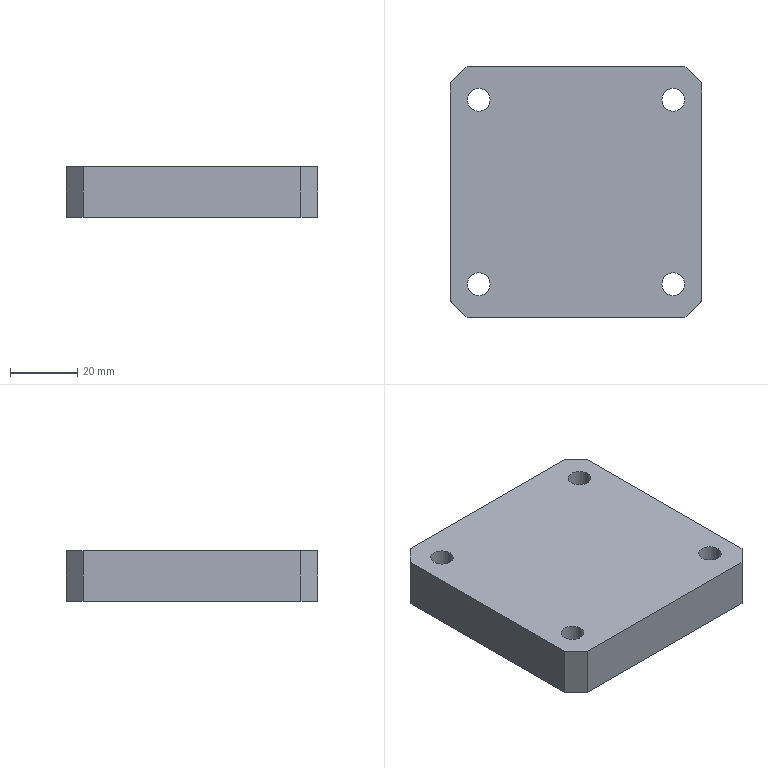Part | SolidWorks | features Extrusion 1, HoleWzd 1 | 1 solid | 18 faces | box 75 x 75 x 15 mm | volume 81446 mm3 | plane 10 | cylinder 8 | commonest cylinder face diameters 6.8 x8
STEP:
#1=CARTESIAN_POINT('',(-25.6,27.5,0.));
#2=VERTEX_POINT('',#1);
#3=CARTESIAN_POINT('',(-32.4,27.5,0.));
#4=VERTEX_POINT('',#3);
#5=CARTESIAN_POINT('',(-29.,27.5,0.));
#6=DIRECTION('',(0.,0.,-1.));
#7=DIRECTION('',(-1.,0.,0.));
#8=AXIS2_PLACEMENT_3D('',#5,#6,#7);
#9=CIRCLE('',#8,3.4);
#10=EDGE_CURVE('',#2,#4,#9,.T.);
#11=ORIENTED_EDGE('',*,*,#10,.T.);
#12=CARTESIAN_POINT('',(-32.4,27.5,15.));
#13=VERTEX_POINT('',#12);
#14=CARTESIAN_POINT('',(-32.4,27.5,15.));
#15=DIRECTION('',(0.,0.,1.));
#16=VECTOR('',#15,1000.);
#17=LINE('',#14,#16);
#18=EDGE_CURVE('',#4,#13,#17,.T.);
#19=ORIENTED_EDGE('',*,*,#18,.T.);
#20=CARTESIAN_POINT('',(-25.6,27.5,15.));
#21=VERTEX_POINT('',#20);
#22=CARTESIAN_POINT('',(-29.,27.5,15.));
#23=DIRECTION('',(0.,0.,1.));
#24=DIRECTION('',(1.,0.,0.));
#25=AXIS2_PLACEMENT_3D('',#22,#23,#24);
#26=CIRCLE('',#25,3.4);
#27=EDGE_CURVE('',#13,#21,#26,.T.);
#28=ORIENTED_EDGE('',*,*,#27,.T.);
#29=CARTESIAN_POINT('',(-25.6,27.5,15.));
#30=DIRECTION('',(0.,0.,1.));
#31=VECTOR('',#30,1000.);
#32=LINE('',#29,#31);
#33=EDGE_CURVE('',#2,#21,#32,.T.);
#34=ORIENTED_EDGE('',*,*,#33,.F.);
#35=EDGE_LOOP('',(#11,#19,#28,#34));
#36=FACE_OUTER_BOUND('',#35,.T.);
#37=CARTESIAN_POINT('',(-29.,27.5,15.));
#38=DIRECTION('',(0.,0.,1.));
#39=DIRECTION('',(1.,0.,0.));
#40=AXIS2_PLACEMENT_3D('',#37,#38,#39);
#41=CYLINDRICAL_SURFACE('',#40,3.4);
#42=ADVANCED_FACE('',(#36),#41,.F.);
#43=CARTESIAN_POINT('',(32.4,27.5,0.));
#44=VERTEX_POINT('',#43);
#45=CARTESIAN_POINT('',(25.6,27.5,0.));
#46=VERTEX_POINT('',#45);
#47=CARTESIAN_POINT('',(29.,27.5,0.));
#48=DIRECTION('',(0.,0.,-1.));
#49=DIRECTION('',(-1.,0.,0.));
#50=AXIS2_PLACEMENT_3D('',#47,#48,#49);
#51=CIRCLE('',#50,3.4);
#52=EDGE_CURVE('',#44,#46,#51,.T.);
#53=ORIENTED_EDGE('',*,*,#52,.T.);
#54=CARTESIAN_POINT('',(25.6,27.5,15.));
#55=VERTEX_POINT('',#54);
#56=CARTESIAN_POINT('',(25.6,27.5,15.));
#57=DIRECTION('',(0.,0.,1.));
#58=VECTOR('',#57,1000.);
#59=LINE('',#56,#58);
#60=EDGE_CURVE('',#46,#55,#59,.T.);
#61=ORIENTED_EDGE('',*,*,#60,.T.);
#62=CARTESIAN_POINT('',(32.4,27.5,15.));
#63=VERTEX_POINT('',#62);
#64=CARTESIAN_POINT('',(29.,27.5,15.));
#65=DIRECTION('',(0.,0.,1.));
#66=DIRECTION('',(1.,0.,0.));
#67=AXIS2_PLACEMENT_3D('',#64,#65,#66);
#68=CIRCLE('',#67,3.4);
#69=EDGE_CURVE('',#55,#63,#68,.T.);
#70=ORIENTED_EDGE('',*,*,#69,.T.);
#71=CARTESIAN_POINT('',(32.4,27.5,15.));
#72=DIRECTION('',(0.,0.,1.));
#73=VECTOR('',#72,1000.);
#74=LINE('',#71,#73);
#75=EDGE_CURVE('',#44,#63,#74,.T.);
#76=ORIENTED_EDGE('',*,*,#75,.F.);
#77=EDGE_LOOP('',(#53,#61,#70,#76));
#78=FACE_OUTER_BOUND('',#77,.T.);
#79=CARTESIAN_POINT('',(29.,27.5,15.));
#80=DIRECTION('',(0.,0.,1.));
#81=DIRECTION('',(1.,0.,0.));
#82=AXIS2_PLACEMENT_3D('',#79,#80,#81);
#83=CYLINDRICAL_SURFACE('',#82,3.4);
#84=ADVANCED_FACE('',(#78),#83,.F.);
#85=CARTESIAN_POINT('',(32.4,-27.5,0.));
#86=VERTEX_POINT('',#85);
#87=CARTESIAN_POINT('',(25.6,-27.5,0.));
#88=VERTEX_POINT('',#87);
#89=CARTESIAN_POINT('',(29.,-27.5,0.));
#90=DIRECTION('',(0.,0.,-1.));
#91=DIRECTION('',(-1.,0.,0.));
#92=AXIS2_PLACEMENT_3D('',#89,#90,#91);
#93=CIRCLE('',#92,3.4);
#94=EDGE_CURVE('',#86,#88,#93,.T.);
#95=ORIENTED_EDGE('',*,*,#94,.T.);
#96=CARTESIAN_POINT('',(25.6,-27.5,15.));
#97=VERTEX_POINT('',#96);
#98=CARTESIAN_POINT('',(25.6,-27.5,15.));
#99=DIRECTION('',(0.,0.,1.));
#100=VECTOR('',#99,1000.);
#101=LINE('',#98,#100);
#102=EDGE_CURVE('',#88,#97,#101,.T.);
#103=ORIENTED_EDGE('',*,*,#102,.T.);
#104=CARTESIAN_POINT('',(32.4,-27.5,15.));
#105=VERTEX_POINT('',#104);
#106=CARTESIAN_POINT('',(29.,-27.5,15.));
#107=DIRECTION('',(0.,0.,1.));
#108=DIRECTION('',(1.,0.,0.));
#109=AXIS2_PLACEMENT_3D('',#106,#107,#108);
#110=CIRCLE('',#109,3.4);
#111=EDGE_CURVE('',#97,#105,#110,.T.);
#112=ORIENTED_EDGE('',*,*,#111,.T.);
#113=CARTESIAN_POINT('',(32.4,-27.5,15.));
#114=DIRECTION('',(0.,0.,1.));
#115=VECTOR('',#114,1000.);
#116=LINE('',#113,#115);
#117=EDGE_CURVE('',#86,#105,#116,.T.);
#118=ORIENTED_EDGE('',*,*,#117,.F.);
#119=EDGE_LOOP('',(#95,#103,#112,#118));
#120=FACE_OUTER_BOUND('',#119,.T.);
#121=CARTESIAN_POINT('',(29.,-27.5,15.));
#122=DIRECTION('',(0.,0.,1.));
#123=DIRECTION('',(1.,0.,0.));
#124=AXIS2_PLACEMENT_3D('',#121,#122,#123);
#125=CYLINDRICAL_SURFACE('',#124,3.4);
#126=ADVANCED_FACE('',(#120),#125,.F.);
#127=CARTESIAN_POINT('',(-25.6,-27.5,0.));
#128=VERTEX_POINT('',#127);
#129=CARTESIAN_POINT('',(-32.4,-27.5,0.));
#130=VERTEX_POINT('',#129);
#131=CARTESIAN_POINT('',(-29.,-27.5,0.));
#132=DIRECTION('',(0.,0.,-1.));
#133=DIRECTION('',(-1.,0.,0.));
#134=AXIS2_PLACEMENT_3D('',#131,#132,#133);
#135=CIRCLE('',#134,3.4);
#136=EDGE_CURVE('',#128,#130,#135,.T.);
#137=ORIENTED_EDGE('',*,*,#136,.T.);
#138=CARTESIAN_POINT('',(-32.4,-27.5,15.));
#139=VERTEX_POINT('',#138);
#140=CARTESIAN_POINT('',(-32.4,-27.5,15.));
#141=DIRECTION('',(0.,0.,1.));
#142=VECTOR('',#141,1000.);
#143=LINE('',#140,#142);
#144=EDGE_CURVE('',#130,#139,#143,.T.);
#145=ORIENTED_EDGE('',*,*,#144,.T.);
#146=CARTESIAN_POINT('',(-25.6,-27.5,15.));
#147=VERTEX_POINT('',#146);
#148=CARTESIAN_POINT('',(-29.,-27.5,15.));
#149=DIRECTION('',(0.,0.,1.));
#150=DIRECTION('',(1.,0.,0.));
#151=AXIS2_PLACEMENT_3D('',#148,#149,#150);
#152=CIRCLE('',#151,3.4);
#153=EDGE_CURVE('',#139,#147,#152,.T.);
#154=ORIENTED_EDGE('',*,*,#153,.T.);
#155=CARTESIAN_POINT('',(-25.6,-27.5,15.));
#156=DIRECTION('',(0.,0.,1.));
#157=VECTOR('',#156,1000.);
#158=LINE('',#155,#157);
#159=EDGE_CURVE('',#128,#147,#158,.T.);
#160=ORIENTED_EDGE('',*,*,#159,.F.);
#161=EDGE_LOOP('',(#137,#145,#154,#160));
#162=FACE_OUTER_BOUND('',#161,.T.);
#163=CARTESIAN_POINT('',(-29.,-27.5,15.));
#164=DIRECTION('',(0.,0.,1.));
#165=DIRECTION('',(1.,0.,0.));
#166=AXIS2_PLACEMENT_3D('',#163,#164,#165);
#167=CYLINDRICAL_SURFACE('',#166,3.4);
#168=ADVANCED_FACE('',(#162),#167,.F.);
#169=CARTESIAN_POINT('',(32.5,37.5,0.));
#170=VERTEX_POINT('',#169);
#171=CARTESIAN_POINT('',(-32.5,37.5,0.));
#172=VERTEX_POINT('',#171);
#173=CARTESIAN_POINT('',(-32.5,37.5,0.));
#174=DIRECTION('',(-1.,0.,0.));
#175=VECTOR('',#174,1000.);
#176=LINE('',#173,#175);
#177=EDGE_CURVE('',#170,#172,#176,.T.);
#178=ORIENTED_EDGE('',*,*,#177,.T.);
#179=CARTESIAN_POINT('',(-32.5,37.5,15.));
#180=VERTEX_POINT('',#179);
#181=CARTESIAN_POINT('',(-32.5,37.5,15.));
#182=DIRECTION('',(0.,0.,-1.));
#183=VECTOR('',#182,1000.);
#184=LINE('',#181,#183);
#185=EDGE_CURVE('',#180,#172,#184,.T.);
#186=ORIENTED_EDGE('',*,*,#185,.F.);
#187=CARTESIAN_POINT('',(32.5,37.5,15.));
#188=VERTEX_POINT('',#187);
#189=CARTESIAN_POINT('',(-32.5,37.5,15.));
#190=DIRECTION('',(-1.,0.,0.));
#191=VECTOR('',#190,1000.);
#192=LINE('',#189,#191);
#193=EDGE_CURVE('',#188,#180,#192,.T.);
#194=ORIENTED_EDGE('',*,*,#193,.F.);
#195=CARTESIAN_POINT('',(32.5,37.5,15.));
#196=DIRECTION('',(0.,0.,-1.));
#197=VECTOR('',#196,1000.);
#198=LINE('',#195,#197);
#199=EDGE_CURVE('',#188,#170,#198,.T.);
#200=ORIENTED_EDGE('',*,*,#199,.T.);
#201=EDGE_LOOP('',(#178,#186,#194,#200));
#202=FACE_OUTER_BOUND('',#201,.T.);
#203=CARTESIAN_POINT('',(-32.5,37.5,15.));
#204=DIRECTION('',(0.,-1.,0.));
#205=DIRECTION('',(0.,0.,-1.));
#206=AXIS2_PLACEMENT_3D('',#203,#204,#205);
#207=PLANE('',#206);
#208=ADVANCED_FACE('',(#202),#207,.F.);
#209=CARTESIAN_POINT('',(-37.5,32.5,0.));
#210=VERTEX_POINT('',#209);
#211=CARTESIAN_POINT('',(-37.5,32.5,0.));
#212=DIRECTION('',(-0.7071,-0.7071,0.));
#213=VECTOR('',#212,1000.);
#214=LINE('',#211,#213);
#215=EDGE_CURVE('',#172,#210,#214,.T.);
#216=ORIENTED_EDGE('',*,*,#215,.T.);
#217=CARTESIAN_POINT('',(-37.5,32.5,15.));
#218=VERTEX_POINT('',#217);
#219=CARTESIAN_POINT('',(-37.5,32.5,15.));
#220=DIRECTION('',(0.,0.,-1.));
#221=VECTOR('',#220,1000.);
#222=LINE('',#219,#221);
#223=EDGE_CURVE('',#218,#210,#222,.T.);
#224=ORIENTED_EDGE('',*,*,#223,.F.);
#225=CARTESIAN_POINT('',(-37.5,32.5,15.));
#226=DIRECTION('',(-0.7071,-0.7071,0.));
#227=VECTOR('',#226,1000.);
#228=LINE('',#225,#227);
#229=EDGE_CURVE('',#180,#218,#228,.T.);
#230=ORIENTED_EDGE('',*,*,#229,.F.);
#231=ORIENTED_EDGE('',*,*,#185,.T.);
#232=EDGE_LOOP('',(#216,#224,#230,#231));
#233=FACE_OUTER_BOUND('',#232,.T.);
#234=CARTESIAN_POINT('',(-37.5,32.5,15.));
#235=DIRECTION('',(0.7071,-0.7071,0.));
#236=DIRECTION('',(0.7071,0.7071,0.));
#237=AXIS2_PLACEMENT_3D('',#234,#235,#236);
#238=PLANE('',#237);
#239=ADVANCED_FACE('',(#233),#238,.F.);
#240=CARTESIAN_POINT('',(-37.5,-32.5,0.));
#241=VERTEX_POINT('',#240);
#242=CARTESIAN_POINT('',(-37.5,32.5,0.));
#243=DIRECTION('',(0.,-1.,0.));
#244=VECTOR('',#243,1000.);
#245=LINE('',#242,#244);
#246=EDGE_CURVE('',#210,#241,#245,.T.);
#247=ORIENTED_EDGE('',*,*,#246,.T.);
#248=CARTESIAN_POINT('',(-37.5,-32.5,15.));
#249=VERTEX_POINT('',#248);
#250=CARTESIAN_POINT('',(-37.5,-32.5,15.));
#251=DIRECTION('',(0.,0.,-1.));
#252=VECTOR('',#251,1000.);
#253=LINE('',#250,#252);
#254=EDGE_CURVE('',#249,#241,#253,.T.);
#255=ORIENTED_EDGE('',*,*,#254,.F.);
#256=CARTESIAN_POINT('',(-37.5,32.5,15.));
#257=DIRECTION('',(0.,-1.,0.));
#258=VECTOR('',#257,1000.);
#259=LINE('',#256,#258);
#260=EDGE_CURVE('',#218,#249,#259,.T.);
#261=ORIENTED_EDGE('',*,*,#260,.F.);
#262=ORIENTED_EDGE('',*,*,#223,.T.);
#263=EDGE_LOOP('',(#247,#255,#261,#262));
#264=FACE_OUTER_BOUND('',#263,.T.);
#265=CARTESIAN_POINT('',(-37.5,32.5,15.));
#266=DIRECTION('',(1.,0.,0.));
#267=DIRECTION('',(0.,0.,-1.));
#268=AXIS2_PLACEMENT_3D('',#265,#266,#267);
#269=PLANE('',#268);
#270=ADVANCED_FACE('',(#264),#269,.F.);
#271=CARTESIAN_POINT('',(-32.5,-37.5,0.));
#272=VERTEX_POINT('',#271);
#273=CARTESIAN_POINT('',(-37.5,-32.5,0.));
#274=DIRECTION('',(0.7071,-0.7071,0.));
#275=VECTOR('',#274,1000.);
#276=LINE('',#273,#275);
#277=EDGE_CURVE('',#241,#272,#276,.T.);
#278=ORIENTED_EDGE('',*,*,#277,.T.);
#279=CARTESIAN_POINT('',(-32.5,-37.5,15.));
#280=VERTEX_POINT('',#279);
#281=CARTESIAN_POINT('',(-32.5,-37.5,15.));
#282=DIRECTION('',(0.,0.,-1.));
#283=VECTOR('',#282,1000.);
#284=LINE('',#281,#283);
#285=EDGE_CURVE('',#280,#272,#284,.T.);
#286=ORIENTED_EDGE('',*,*,#285,.F.);
#287=CARTESIAN_POINT('',(-37.5,-32.5,15.));
#288=DIRECTION('',(0.7071,-0.7071,0.));
#289=VECTOR('',#288,1000.);
#290=LINE('',#287,#289);
#291=EDGE_CURVE('',#249,#280,#290,.T.);
#292=ORIENTED_EDGE('',*,*,#291,.F.);
#293=ORIENTED_EDGE('',*,*,#254,.T.);
#294=EDGE_LOOP('',(#278,#286,#292,#293));
#295=FACE_OUTER_BOUND('',#294,.T.);
#296=CARTESIAN_POINT('',(-37.5,-32.5,15.));
#297=DIRECTION('',(0.7071,0.7071,0.));
#298=DIRECTION('',(-0.7071,0.7071,0.));
#299=AXIS2_PLACEMENT_3D('',#296,#297,#298);
#300=PLANE('',#299);
#301=ADVANCED_FACE('',(#295),#300,.F.);
#302=CARTESIAN_POINT('',(32.5,-37.5,0.));
#303=VERTEX_POINT('',#302);
#304=CARTESIAN_POINT('',(-32.5,-37.5,0.));
#305=DIRECTION('',(1.,0.,0.));
#306=VECTOR('',#305,1000.);
#307=LINE('',#304,#306);
#308=EDGE_CURVE('',#272,#303,#307,.T.);
#309=ORIENTED_EDGE('',*,*,#308,.T.);
#310=CARTESIAN_POINT('',(32.5,-37.5,15.));
#311=VERTEX_POINT('',#310);
#312=CARTESIAN_POINT('',(32.5,-37.5,15.));
#313=DIRECTION('',(0.,0.,-1.));
#314=VECTOR('',#313,1000.);
#315=LINE('',#312,#314);
#316=EDGE_CURVE('',#311,#303,#315,.T.);
#317=ORIENTED_EDGE('',*,*,#316,.F.);
#318=CARTESIAN_POINT('',(-32.5,-37.5,15.));
#319=DIRECTION('',(1.,0.,0.));
#320=VECTOR('',#319,1000.);
#321=LINE('',#318,#320);
#322=EDGE_CURVE('',#280,#311,#321,.T.);
#323=ORIENTED_EDGE('',*,*,#322,.F.);
#324=ORIENTED_EDGE('',*,*,#285,.T.);
#325=EDGE_LOOP('',(#309,#317,#323,#324));
#326=FACE_OUTER_BOUND('',#325,.T.);
#327=CARTESIAN_POINT('',(-32.5,-37.5,15.));
#328=DIRECTION('',(0.,1.,0.));
#329=DIRECTION('',(0.,0.,1.));
#330=AXIS2_PLACEMENT_3D('',#327,#328,#329);
#331=PLANE('',#330);
#332=ADVANCED_FACE('',(#326),#331,.F.);
#333=CARTESIAN_POINT('',(37.5,-32.5,0.));
#334=VERTEX_POINT('',#333);
#335=CARTESIAN_POINT('',(32.5,-37.5,0.));
#336=DIRECTION('',(0.7071,0.7071,0.));
#337=VECTOR('',#336,1000.);
#338=LINE('',#335,#337);
#339=EDGE_CURVE('',#303,#334,#338,.T.);
#340=ORIENTED_EDGE('',*,*,#339,.T.);
#341=CARTESIAN_POINT('',(37.5,-32.5,15.));
#342=VERTEX_POINT('',#341);
#343=CARTESIAN_POINT('',(37.5,-32.5,15.));
#344=DIRECTION('',(0.,0.,-1.));
#345=VECTOR('',#344,1000.);
#346=LINE('',#343,#345);
#347=EDGE_CURVE('',#342,#334,#346,.T.);
#348=ORIENTED_EDGE('',*,*,#347,.F.);
#349=CARTESIAN_POINT('',(32.5,-37.5,15.));
#350=DIRECTION('',(0.7071,0.7071,0.));
#351=VECTOR('',#350,1000.);
#352=LINE('',#349,#351);
#353=EDGE_CURVE('',#311,#342,#352,.T.);
#354=ORIENTED_EDGE('',*,*,#353,.F.);
#355=ORIENTED_EDGE('',*,*,#316,.T.);
#356=EDGE_LOOP('',(#340,#348,#354,#355));
#357=FACE_OUTER_BOUND('',#356,.T.);
#358=CARTESIAN_POINT('',(32.5,-37.5,15.));
#359=DIRECTION('',(-0.7071,0.7071,0.));
#360=DIRECTION('',(-0.7071,-0.7071,0.));
#361=AXIS2_PLACEMENT_3D('',#358,#359,#360);
#362=PLANE('',#361);
#363=ADVANCED_FACE('',(#357),#362,.F.);
#364=CARTESIAN_POINT('',(37.5,32.5,0.));
#365=VERTEX_POINT('',#364);
#366=CARTESIAN_POINT('',(37.5,32.5,0.));
#367=DIRECTION('',(0.,1.,0.));
#368=VECTOR('',#367,1000.);
#369=LINE('',#366,#368);
#370=EDGE_CURVE('',#334,#365,#369,.T.);
#371=ORIENTED_EDGE('',*,*,#370,.T.);
#372=CARTESIAN_POINT('',(37.5,32.5,15.));
#373=VERTEX_POINT('',#372);
#374=CARTESIAN_POINT('',(37.5,32.5,15.));
#375=DIRECTION('',(0.,0.,-1.));
#376=VECTOR('',#375,1000.);
#377=LINE('',#374,#376);
#378=EDGE_CURVE('',#373,#365,#377,.T.);
#379=ORIENTED_EDGE('',*,*,#378,.F.);
#380=CARTESIAN_POINT('',(37.5,32.5,15.));
#381=DIRECTION('',(0.,1.,0.));
#382=VECTOR('',#381,1000.);
#383=LINE('',#380,#382);
#384=EDGE_CURVE('',#342,#373,#383,.T.);
#385=ORIENTED_EDGE('',*,*,#384,.F.);
#386=ORIENTED_EDGE('',*,*,#347,.T.);
#387=EDGE_LOOP('',(#371,#379,#385,#386));
#388=FACE_OUTER_BOUND('',#387,.T.);
#389=CARTESIAN_POINT('',(37.5,32.5,15.));
#390=DIRECTION('',(-1.,0.,0.));
#391=DIRECTION('',(0.,-1.,0.));
#392=AXIS2_PLACEMENT_3D('',#389,#390,#391);
#393=PLANE('',#392);
#394=ADVANCED_FACE('',(#388),#393,.F.);
#395=CARTESIAN_POINT('',(32.5,37.5,0.));
#396=DIRECTION('',(-0.7071,0.7071,0.));
#397=VECTOR('',#396,1000.);
#398=LINE('',#395,#397);
#399=EDGE_CURVE('',#365,#170,#398,.T.);
#400=ORIENTED_EDGE('',*,*,#399,.T.);
#401=ORIENTED_EDGE('',*,*,#199,.F.);
#402=CARTESIAN_POINT('',(32.5,37.5,15.));
#403=DIRECTION('',(-0.7071,0.7071,0.));
#404=VECTOR('',#403,1000.);
#405=LINE('',#402,#404);
#406=EDGE_CURVE('',#373,#188,#405,.T.);
#407=ORIENTED_EDGE('',*,*,#406,.F.);
#408=ORIENTED_EDGE('',*,*,#378,.T.);
#409=EDGE_LOOP('',(#400,#401,#407,#408));
#410=FACE_OUTER_BOUND('',#409,.T.);
#411=CARTESIAN_POINT('',(32.5,37.5,15.));
#412=DIRECTION('',(-0.7071,-0.7071,0.));
#413=DIRECTION('',(0.7071,-0.7071,0.));
#414=AXIS2_PLACEMENT_3D('',#411,#412,#413);
#415=PLANE('',#414);
#416=ADVANCED_FACE('',(#410),#415,.F.);
#417=CARTESIAN_POINT('',(-29.,27.5,15.));
#418=DIRECTION('',(0.,0.,1.));
#419=DIRECTION('',(1.,0.,0.));
#420=AXIS2_PLACEMENT_3D('',#417,#418,#419);
#421=CIRCLE('',#420,3.4);
#422=EDGE_CURVE('',#21,#13,#421,.T.);
#423=ORIENTED_EDGE('',*,*,#422,.F.);
#424=ORIENTED_EDGE('',*,*,#27,.F.);
#425=EDGE_LOOP('',(#423,#424));
#426=FACE_BOUND('',#425,.T.);
#427=CARTESIAN_POINT('',(29.,27.5,15.));
#428=DIRECTION('',(0.,0.,1.));
#429=DIRECTION('',(1.,0.,0.));
#430=AXIS2_PLACEMENT_3D('',#427,#428,#429);
#431=CIRCLE('',#430,3.4);
#432=EDGE_CURVE('',#63,#55,#431,.T.);
#433=ORIENTED_EDGE('',*,*,#432,.F.);
#434=ORIENTED_EDGE('',*,*,#69,.F.);
#435=EDGE_LOOP('',(#433,#434));
#436=FACE_BOUND('',#435,.T.);
#437=CARTESIAN_POINT('',(29.,-27.5,15.));
#438=DIRECTION('',(0.,0.,1.));
#439=DIRECTION('',(1.,0.,0.));
#440=AXIS2_PLACEMENT_3D('',#437,#438,#439);
#441=CIRCLE('',#440,3.4);
#442=EDGE_CURVE('',#105,#97,#441,.T.);
#443=ORIENTED_EDGE('',*,*,#442,.F.);
#444=ORIENTED_EDGE('',*,*,#111,.F.);
#445=EDGE_LOOP('',(#443,#444));
#446=FACE_BOUND('',#445,.T.);
#447=CARTESIAN_POINT('',(-29.,-27.5,15.));
#448=DIRECTION('',(0.,0.,1.));
#449=DIRECTION('',(1.,0.,0.));
#450=AXIS2_PLACEMENT_3D('',#447,#448,#449);
#451=CIRCLE('',#450,3.4);
#452=EDGE_CURVE('',#147,#139,#451,.T.);
#453=ORIENTED_EDGE('',*,*,#452,.F.);
#454=ORIENTED_EDGE('',*,*,#153,.F.);
#455=EDGE_LOOP('',(#453,#454));
#456=FACE_BOUND('',#455,.T.);
#457=ORIENTED_EDGE('',*,*,#193,.T.);
#458=ORIENTED_EDGE('',*,*,#229,.T.);
#459=ORIENTED_EDGE('',*,*,#260,.T.);
#460=ORIENTED_EDGE('',*,*,#291,.T.);
#461=ORIENTED_EDGE('',*,*,#322,.T.);
#462=ORIENTED_EDGE('',*,*,#353,.T.);
#463=ORIENTED_EDGE('',*,*,#384,.T.);
#464=ORIENTED_EDGE('',*,*,#406,.T.);
#465=EDGE_LOOP('',(#457,#458,#459,#460,#461,#462,#463,#464));
#466=FACE_OUTER_BOUND('',#465,.T.);
#467=CARTESIAN_POINT('',(0.,0.,15.));
#468=DIRECTION('',(0.,0.,-1.));
#469=DIRECTION('',(-1.,0.,0.));
#470=AXIS2_PLACEMENT_3D('',#467,#468,#469);
#471=PLANE('',#470);
#472=ADVANCED_FACE('',(#426,#436,#446,#456,#466),#471,.F.);
#473=ORIENTED_EDGE('',*,*,#10,.F.);
#474=CARTESIAN_POINT('',(-29.,27.5,0.));
#475=DIRECTION('',(0.,0.,-1.));
#476=DIRECTION('',(-1.,0.,0.));
#477=AXIS2_PLACEMENT_3D('',#474,#475,#476);
#478=CIRCLE('',#477,3.4);
#479=EDGE_CURVE('',#4,#2,#478,.T.);
#480=ORIENTED_EDGE('',*,*,#479,.F.);
#481=EDGE_LOOP('',(#473,#480));
#482=FACE_BOUND('',#481,.T.);
#483=ORIENTED_EDGE('',*,*,#52,.F.);
#484=CARTESIAN_POINT('',(29.,27.5,0.));
#485=DIRECTION('',(0.,0.,-1.));
#486=DIRECTION('',(-1.,0.,0.));
#487=AXIS2_PLACEMENT_3D('',#484,#485,#486);
#488=CIRCLE('',#487,3.4);
#489=EDGE_CURVE('',#46,#44,#488,.T.);
#490=ORIENTED_EDGE('',*,*,#489,.F.);
#491=EDGE_LOOP('',(#483,#490));
#492=FACE_BOUND('',#491,.T.);
#493=ORIENTED_EDGE('',*,*,#94,.F.);
#494=CARTESIAN_POINT('',(29.,-27.5,0.));
#495=DIRECTION('',(0.,0.,-1.));
#496=DIRECTION('',(-1.,0.,0.));
#497=AXIS2_PLACEMENT_3D('',#494,#495,#496);
#498=CIRCLE('',#497,3.4);
#499=EDGE_CURVE('',#88,#86,#498,.T.);
#500=ORIENTED_EDGE('',*,*,#499,.F.);
#501=EDGE_LOOP('',(#493,#500));
#502=FACE_BOUND('',#501,.T.);
#503=ORIENTED_EDGE('',*,*,#136,.F.);
#504=CARTESIAN_POINT('',(-29.,-27.5,0.));
#505=DIRECTION('',(0.,0.,-1.));
#506=DIRECTION('',(-1.,0.,0.));
#507=AXIS2_PLACEMENT_3D('',#504,#505,#506);
#508=CIRCLE('',#507,3.4);
#509=EDGE_CURVE('',#130,#128,#508,.T.);
#510=ORIENTED_EDGE('',*,*,#509,.F.);
#511=EDGE_LOOP('',(#503,#510));
#512=FACE_BOUND('',#511,.T.);
#513=ORIENTED_EDGE('',*,*,#177,.F.);
#514=ORIENTED_EDGE('',*,*,#399,.F.);
#515=ORIENTED_EDGE('',*,*,#370,.F.);
#516=ORIENTED_EDGE('',*,*,#339,.F.);
#517=ORIENTED_EDGE('',*,*,#308,.F.);
#518=ORIENTED_EDGE('',*,*,#277,.F.);
#519=ORIENTED_EDGE('',*,*,#246,.F.);
#520=ORIENTED_EDGE('',*,*,#215,.F.);
#521=EDGE_LOOP('',(#513,#514,#515,#516,#517,#518,#519,#520));
#522=FACE_OUTER_BOUND('',#521,.T.);
#523=CARTESIAN_POINT('',(0.,0.,0.));
#524=DIRECTION('',(0.,0.,-1.));
#525=DIRECTION('',(-1.,0.,0.));
#526=AXIS2_PLACEMENT_3D('',#523,#524,#525);
#527=PLANE('',#526);
#528=ADVANCED_FACE('',(#482,#492,#502,#512,#522),#527,.T.);
#529=ORIENTED_EDGE('',*,*,#144,.F.);
#530=ORIENTED_EDGE('',*,*,#509,.T.);
#531=ORIENTED_EDGE('',*,*,#159,.T.);
#532=ORIENTED_EDGE('',*,*,#452,.T.);
#533=EDGE_LOOP('',(#529,#530,#531,#532));
#534=FACE_OUTER_BOUND('',#533,.T.);
#535=CARTESIAN_POINT('',(-29.,-27.5,15.));
#536=DIRECTION('',(0.,0.,1.));
#537=DIRECTION('',(1.,0.,0.));
#538=AXIS2_PLACEMENT_3D('',#535,#536,#537);
#539=CYLINDRICAL_SURFACE('',#538,3.4);
#540=ADVANCED_FACE('',(#534),#539,.F.);
#541=ORIENTED_EDGE('',*,*,#102,.F.);
#542=ORIENTED_EDGE('',*,*,#499,.T.);
#543=ORIENTED_EDGE('',*,*,#117,.T.);
#544=ORIENTED_EDGE('',*,*,#442,.T.);
#545=EDGE_LOOP('',(#541,#542,#543,#544));
#546=FACE_OUTER_BOUND('',#545,.T.);
#547=CARTESIAN_POINT('',(29.,-27.5,15.));
#548=DIRECTION('',(0.,0.,1.));
#549=DIRECTION('',(1.,0.,0.));
#550=AXIS2_PLACEMENT_3D('',#547,#548,#549);
#551=CYLINDRICAL_SURFACE('',#550,3.4);
#552=ADVANCED_FACE('',(#546),#551,.F.);
#553=ORIENTED_EDGE('',*,*,#60,.F.);
#554=ORIENTED_EDGE('',*,*,#489,.T.);
#555=ORIENTED_EDGE('',*,*,#75,.T.);
#556=ORIENTED_EDGE('',*,*,#432,.T.);
#557=EDGE_LOOP('',(#553,#554,#555,#556));
#558=FACE_OUTER_BOUND('',#557,.T.);
#559=CARTESIAN_POINT('',(29.,27.5,15.));
#560=DIRECTION('',(0.,0.,1.));
#561=DIRECTION('',(1.,0.,0.));
#562=AXIS2_PLACEMENT_3D('',#559,#560,#561);
#563=CYLINDRICAL_SURFACE('',#562,3.4);
#564=ADVANCED_FACE('',(#558),#563,.F.);
#565=ORIENTED_EDGE('',*,*,#18,.F.);
#566=ORIENTED_EDGE('',*,*,#479,.T.);
#567=ORIENTED_EDGE('',*,*,#33,.T.);
#568=ORIENTED_EDGE('',*,*,#422,.T.);
#569=EDGE_LOOP('',(#565,#566,#567,#568));
#570=FACE_OUTER_BOUND('',#569,.T.);
#571=CARTESIAN_POINT('',(-29.,27.5,15.));
#572=DIRECTION('',(0.,0.,1.));
#573=DIRECTION('',(1.,0.,0.));
#574=AXIS2_PLACEMENT_3D('',#571,#572,#573);
#575=CYLINDRICAL_SURFACE('',#574,3.4);
#576=ADVANCED_FACE('',(#570),#575,.F.);
#577=CLOSED_SHELL('',(#42,#84,#126,#168,#208,#239,#270,#301,#332,#363,#394,#416,#472,#528,#540,#552,#564,#576));
#578=MANIFOLD_SOLID_BREP('',#577);
#579=CARTESIAN_POINT('',(0.,0.,0.));
#580=DIRECTION('',(0.,0.,1.));
#581=DIRECTION('',(1.,0.,0.));
#582=AXIS2_PLACEMENT_3D('',#579,#580,#581);
#583=(LENGTH_UNIT()NAMED_UNIT(*)SI_UNIT(.MILLI.,.METRE.));
#584=UNCERTAINTY_MEASURE_WITH_UNIT(LENGTH_MEASURE(0.00001),#583,'','');
#585=(NAMED_UNIT(*)PLANE_ANGLE_UNIT()SI_UNIT($,.RADIAN.));
#586=(NAMED_UNIT(*)SI_UNIT($,.STERADIAN.)SOLID_ANGLE_UNIT());
#587=(GEOMETRIC_REPRESENTATION_CONTEXT(3)GLOBAL_UNCERTAINTY_ASSIGNED_CONTEXT((#584))GLOBAL_UNIT_ASSIGNED_CONTEXT((#583,#585,#586))REPRESENTATION_CONTEXT('',''));
#588=ADVANCED_BREP_SHAPE_REPRESENTATION('',(#578,#582),#587);